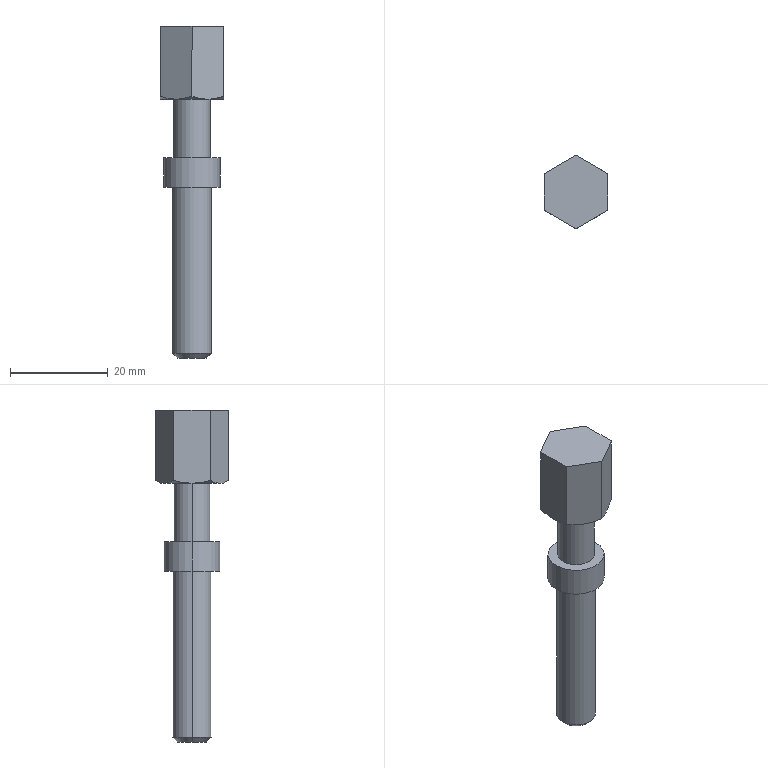Part | SolidWorks | features BaseBody 1 | 1 solid | 25 faces | box 13 x 15.011 x 68 mm | volume 5094 mm3 | plane 11 | cone 8 | cylinder 6 | commonest cylinder face diameters 7.5 x2 8 x2 11.5 x2
STEP:
#1=CARTESIAN_POINT('',(-4.,0.,-33.));
#2=VERTEX_POINT('',#1);
#3=CARTESIAN_POINT('',(4.,0.,-33.));
#4=VERTEX_POINT('',#3);
#5=CARTESIAN_POINT('',(0.,0.,-33.));
#6=DIRECTION('',(0.,0.,-1.));
#7=DIRECTION('',(-1.,0.,0.));
#8=AXIS2_PLACEMENT_3D('',#5,#6,#7);
#9=CIRCLE('',#8,4.);
#10=EDGE_CURVE('',#2,#4,#9,.T.);
#11=ORIENTED_EDGE('',*,*,#10,.T.);
#12=CARTESIAN_POINT('',(4.,0.,-67.));
#13=VERTEX_POINT('',#12);
#14=CARTESIAN_POINT('',(4.,0.,-68.));
#15=DIRECTION('',(0.,0.,-1.));
#16=VECTOR('',#15,1000.);
#17=LINE('',#14,#16);
#18=EDGE_CURVE('',#4,#13,#17,.T.);
#19=ORIENTED_EDGE('',*,*,#18,.T.);
#20=CARTESIAN_POINT('',(-4.,0.,-67.));
#21=VERTEX_POINT('',#20);
#22=CARTESIAN_POINT('',(0.,0.,-67.));
#23=DIRECTION('',(0.,0.,1.));
#24=DIRECTION('',(-1.,0.,0.));
#25=AXIS2_PLACEMENT_3D('',#22,#23,#24);
#26=CIRCLE('',#25,4.);
#27=EDGE_CURVE('',#13,#21,#26,.T.);
#28=ORIENTED_EDGE('',*,*,#27,.T.);
#29=CARTESIAN_POINT('',(-4.,0.,-68.));
#30=DIRECTION('',(0.,0.,-1.));
#31=VECTOR('',#30,1000.);
#32=LINE('',#29,#31);
#33=EDGE_CURVE('',#2,#21,#32,.T.);
#34=ORIENTED_EDGE('',*,*,#33,.F.);
#35=EDGE_LOOP('',(#11,#19,#28,#34));
#36=FACE_OUTER_BOUND('',#35,.T.);
#37=CARTESIAN_POINT('',(0.,0.,-68.));
#38=DIRECTION('',(0.,0.,-1.));
#39=DIRECTION('',(-1.,0.,0.));
#40=AXIS2_PLACEMENT_3D('',#37,#38,#39);
#41=CYLINDRICAL_SURFACE('',#40,4.);
#42=ADVANCED_FACE('',(#36),#41,.T.);
#43=CARTESIAN_POINT('',(3.,0.,-68.));
#44=VERTEX_POINT('',#43);
#45=CARTESIAN_POINT('',(-3.,0.,-68.));
#46=VERTEX_POINT('',#45);
#47=CARTESIAN_POINT('',(0.,0.,-68.));
#48=DIRECTION('',(0.,0.,1.));
#49=DIRECTION('',(1.,0.,0.));
#50=AXIS2_PLACEMENT_3D('',#47,#48,#49);
#51=CIRCLE('',#50,3.);
#52=EDGE_CURVE('',#44,#46,#51,.T.);
#53=ORIENTED_EDGE('',*,*,#52,.T.);
#54=CARTESIAN_POINT('',(-4.,0.,-67.));
#55=DIRECTION('',(-0.7071,0.,0.7071));
#56=VECTOR('',#55,1000.);
#57=LINE('',#54,#56);
#58=EDGE_CURVE('',#46,#21,#57,.T.);
#59=ORIENTED_EDGE('',*,*,#58,.T.);
#60=ORIENTED_EDGE('',*,*,#27,.F.);
#61=CARTESIAN_POINT('',(4.,0.,-67.));
#62=DIRECTION('',(0.7071,0.,0.7071));
#63=VECTOR('',#62,1000.);
#64=LINE('',#61,#63);
#65=EDGE_CURVE('',#44,#13,#64,.T.);
#66=ORIENTED_EDGE('',*,*,#65,.F.);
#67=EDGE_LOOP('',(#53,#59,#60,#66));
#68=FACE_OUTER_BOUND('',#67,.T.);
#69=CARTESIAN_POINT('',(0.,0.,-67.));
#70=DIRECTION('',(0.,0.,1.));
#71=DIRECTION('',(1.,0.,0.));
#72=AXIS2_PLACEMENT_3D('',#69,#70,#71);
#73=CONICAL_SURFACE('',#72,4.,0.7854);
#74=ADVANCED_FACE('',(#68),#73,.T.);
#75=CARTESIAN_POINT('',(-5.75,0.,-27.));
#76=VERTEX_POINT('',#75);
#77=CARTESIAN_POINT('',(5.75,0.,-27.));
#78=VERTEX_POINT('',#77);
#79=CARTESIAN_POINT('',(0.,0.,-27.));
#80=DIRECTION('',(0.,0.,-1.));
#81=DIRECTION('',(-1.,0.,0.));
#82=AXIS2_PLACEMENT_3D('',#79,#80,#81);
#83=CIRCLE('',#82,5.75);
#84=EDGE_CURVE('',#76,#78,#83,.T.);
#85=ORIENTED_EDGE('',*,*,#84,.T.);
#86=CARTESIAN_POINT('',(5.75,0.,-33.));
#87=VERTEX_POINT('',#86);
#88=CARTESIAN_POINT('',(5.75,0.,-68.));
#89=DIRECTION('',(0.,0.,-1.));
#90=VECTOR('',#89,1000.);
#91=LINE('',#88,#90);
#92=EDGE_CURVE('',#78,#87,#91,.T.);
#93=ORIENTED_EDGE('',*,*,#92,.T.);
#94=CARTESIAN_POINT('',(-5.75,0.,-33.));
#95=VERTEX_POINT('',#94);
#96=CARTESIAN_POINT('',(0.,0.,-33.));
#97=DIRECTION('',(0.,0.,1.));
#98=DIRECTION('',(-1.,0.,0.));
#99=AXIS2_PLACEMENT_3D('',#96,#97,#98);
#100=CIRCLE('',#99,5.75);
#101=EDGE_CURVE('',#87,#95,#100,.T.);
#102=ORIENTED_EDGE('',*,*,#101,.T.);
#103=CARTESIAN_POINT('',(-5.75,0.,-68.));
#104=DIRECTION('',(0.,0.,-1.));
#105=VECTOR('',#104,1000.);
#106=LINE('',#103,#105);
#107=EDGE_CURVE('',#76,#95,#106,.T.);
#108=ORIENTED_EDGE('',*,*,#107,.F.);
#109=EDGE_LOOP('',(#85,#93,#102,#108));
#110=FACE_OUTER_BOUND('',#109,.T.);
#111=CARTESIAN_POINT('',(0.,0.,-68.));
#112=DIRECTION('',(0.,0.,-1.));
#113=DIRECTION('',(-1.,0.,0.));
#114=AXIS2_PLACEMENT_3D('',#111,#112,#113);
#115=CYLINDRICAL_SURFACE('',#114,5.75);
#116=ADVANCED_FACE('',(#110),#115,.T.);
#117=CARTESIAN_POINT('',(-3.75,0.,-15.));
#118=VERTEX_POINT('',#117);
#119=CARTESIAN_POINT('',(3.75,0.,-15.));
#120=VERTEX_POINT('',#119);
#121=CARTESIAN_POINT('',(0.,0.,-15.));
#122=DIRECTION('',(0.,0.,-1.));
#123=DIRECTION('',(-1.,0.,0.));
#124=AXIS2_PLACEMENT_3D('',#121,#122,#123);
#125=CIRCLE('',#124,3.75);
#126=EDGE_CURVE('',#118,#120,#125,.T.);
#127=ORIENTED_EDGE('',*,*,#126,.T.);
#128=CARTESIAN_POINT('',(3.75,0.,-27.));
#129=VERTEX_POINT('',#128);
#130=CARTESIAN_POINT('',(3.75,0.,-68.));
#131=DIRECTION('',(0.,0.,-1.));
#132=VECTOR('',#131,1000.);
#133=LINE('',#130,#132);
#134=EDGE_CURVE('',#120,#129,#133,.T.);
#135=ORIENTED_EDGE('',*,*,#134,.T.);
#136=CARTESIAN_POINT('',(-3.75,0.,-27.));
#137=VERTEX_POINT('',#136);
#138=CARTESIAN_POINT('',(0.,0.,-27.));
#139=DIRECTION('',(0.,0.,1.));
#140=DIRECTION('',(-1.,0.,0.));
#141=AXIS2_PLACEMENT_3D('',#138,#139,#140);
#142=CIRCLE('',#141,3.75);
#143=EDGE_CURVE('',#129,#137,#142,.T.);
#144=ORIENTED_EDGE('',*,*,#143,.T.);
#145=CARTESIAN_POINT('',(-3.75,0.,-68.));
#146=DIRECTION('',(0.,0.,-1.));
#147=VECTOR('',#146,1000.);
#148=LINE('',#145,#147);
#149=EDGE_CURVE('',#118,#137,#148,.T.);
#150=ORIENTED_EDGE('',*,*,#149,.F.);
#151=EDGE_LOOP('',(#127,#135,#144,#150));
#152=FACE_OUTER_BOUND('',#151,.T.);
#153=CARTESIAN_POINT('',(0.,0.,-68.));
#154=DIRECTION('',(0.,0.,-1.));
#155=DIRECTION('',(-1.,0.,0.));
#156=AXIS2_PLACEMENT_3D('',#153,#154,#155);
#157=CYLINDRICAL_SURFACE('',#156,3.75);
#158=ADVANCED_FACE('',(#152),#157,.T.);
#159=ORIENTED_EDGE('',*,*,#18,.F.);
#160=CARTESIAN_POINT('',(0.,0.,-33.));
#161=DIRECTION('',(0.,0.,-1.));
#162=DIRECTION('',(-1.,0.,0.));
#163=AXIS2_PLACEMENT_3D('',#160,#161,#162);
#164=CIRCLE('',#163,4.);
#165=EDGE_CURVE('',#4,#2,#164,.T.);
#166=ORIENTED_EDGE('',*,*,#165,.T.);
#167=ORIENTED_EDGE('',*,*,#33,.T.);
#168=CARTESIAN_POINT('',(0.,0.,-67.));
#169=DIRECTION('',(0.,0.,1.));
#170=DIRECTION('',(-1.,0.,0.));
#171=AXIS2_PLACEMENT_3D('',#168,#169,#170);
#172=CIRCLE('',#171,4.);
#173=EDGE_CURVE('',#21,#13,#172,.T.);
#174=ORIENTED_EDGE('',*,*,#173,.T.);
#175=EDGE_LOOP('',(#159,#166,#167,#174));
#176=FACE_OUTER_BOUND('',#175,.T.);
#177=CARTESIAN_POINT('',(0.,0.,-68.));
#178=DIRECTION('',(0.,0.,-1.));
#179=DIRECTION('',(-1.,0.,0.));
#180=AXIS2_PLACEMENT_3D('',#177,#178,#179);
#181=CYLINDRICAL_SURFACE('',#180,4.);
#182=ADVANCED_FACE('',(#176),#181,.T.);
#183=CARTESIAN_POINT('',(0.,0.,-33.));
#184=DIRECTION('',(0.,0.,1.));
#185=DIRECTION('',(-1.,0.,0.));
#186=AXIS2_PLACEMENT_3D('',#183,#184,#185);
#187=CIRCLE('',#186,5.75);
#188=EDGE_CURVE('',#95,#87,#187,.T.);
#189=ORIENTED_EDGE('',*,*,#188,.F.);
#190=ORIENTED_EDGE('',*,*,#101,.F.);
#191=EDGE_LOOP('',(#189,#190));
#192=FACE_OUTER_BOUND('',#191,.T.);
#193=ORIENTED_EDGE('',*,*,#10,.F.);
#194=ORIENTED_EDGE('',*,*,#165,.F.);
#195=EDGE_LOOP('',(#193,#194));
#196=FACE_BOUND('',#195,.T.);
#197=CARTESIAN_POINT('',(0.,5.75,-33.));
#198=DIRECTION('',(0.,0.,1.));
#199=DIRECTION('',(1.,0.,0.));
#200=AXIS2_PLACEMENT_3D('',#197,#198,#199);
#201=PLANE('',#200);
#202=ADVANCED_FACE('',(#192,#196),#201,.F.);
#203=ORIENTED_EDGE('',*,*,#58,.F.);
#204=CARTESIAN_POINT('',(0.,0.,-68.));
#205=DIRECTION('',(0.,0.,1.));
#206=DIRECTION('',(1.,0.,0.));
#207=AXIS2_PLACEMENT_3D('',#204,#205,#206);
#208=CIRCLE('',#207,3.);
#209=EDGE_CURVE('',#46,#44,#208,.T.);
#210=ORIENTED_EDGE('',*,*,#209,.T.);
#211=ORIENTED_EDGE('',*,*,#65,.T.);
#212=ORIENTED_EDGE('',*,*,#173,.F.);
#213=EDGE_LOOP('',(#203,#210,#211,#212));
#214=FACE_OUTER_BOUND('',#213,.T.);
#215=CARTESIAN_POINT('',(0.,0.,-67.));
#216=DIRECTION('',(0.,0.,1.));
#217=DIRECTION('',(1.,0.,0.));
#218=AXIS2_PLACEMENT_3D('',#215,#216,#217);
#219=CONICAL_SURFACE('',#218,4.,0.7854);
#220=ADVANCED_FACE('',(#214),#219,.T.);
#221=ORIENTED_EDGE('',*,*,#92,.F.);
#222=CARTESIAN_POINT('',(0.,0.,-27.));
#223=DIRECTION('',(0.,0.,-1.));
#224=DIRECTION('',(-1.,0.,0.));
#225=AXIS2_PLACEMENT_3D('',#222,#223,#224);
#226=CIRCLE('',#225,5.75);
#227=EDGE_CURVE('',#78,#76,#226,.T.);
#228=ORIENTED_EDGE('',*,*,#227,.T.);
#229=ORIENTED_EDGE('',*,*,#107,.T.);
#230=ORIENTED_EDGE('',*,*,#188,.T.);
#231=EDGE_LOOP('',(#221,#228,#229,#230));
#232=FACE_OUTER_BOUND('',#231,.T.);
#233=CARTESIAN_POINT('',(0.,0.,-68.));
#234=DIRECTION('',(0.,0.,-1.));
#235=DIRECTION('',(-1.,0.,0.));
#236=AXIS2_PLACEMENT_3D('',#233,#234,#235);
#237=CYLINDRICAL_SURFACE('',#236,5.75);
#238=ADVANCED_FACE('',(#232),#237,.T.);
#239=ORIENTED_EDGE('',*,*,#52,.F.);
#240=ORIENTED_EDGE('',*,*,#209,.F.);
#241=EDGE_LOOP('',(#239,#240));
#242=FACE_OUTER_BOUND('',#241,.T.);
#243=CARTESIAN_POINT('',(0.,3.,-68.));
#244=DIRECTION('',(0.,0.,1.));
#245=DIRECTION('',(1.,0.,0.));
#246=AXIS2_PLACEMENT_3D('',#243,#244,#245);
#247=PLANE('',#246);
#248=ADVANCED_FACE('',(#242),#247,.F.);
#249=CARTESIAN_POINT('',(0.,0.,-27.));
#250=DIRECTION('',(0.,0.,1.));
#251=DIRECTION('',(-1.,0.,0.));
#252=AXIS2_PLACEMENT_3D('',#249,#250,#251);
#253=CIRCLE('',#252,3.75);
#254=EDGE_CURVE('',#137,#129,#253,.T.);
#255=ORIENTED_EDGE('',*,*,#254,.F.);
#256=ORIENTED_EDGE('',*,*,#143,.F.);
#257=EDGE_LOOP('',(#255,#256));
#258=FACE_BOUND('',#257,.T.);
#259=ORIENTED_EDGE('',*,*,#84,.F.);
#260=ORIENTED_EDGE('',*,*,#227,.F.);
#261=EDGE_LOOP('',(#259,#260));
#262=FACE_OUTER_BOUND('',#261,.T.);
#263=CARTESIAN_POINT('',(0.,3.75,-27.));
#264=DIRECTION('',(0.,0.,-1.));
#265=DIRECTION('',(-1.,0.,0.));
#266=AXIS2_PLACEMENT_3D('',#263,#264,#265);
#267=PLANE('',#266);
#268=ADVANCED_FACE('',(#258,#262),#267,.F.);
#269=ORIENTED_EDGE('',*,*,#134,.F.);
#270=CARTESIAN_POINT('',(0.,0.,-15.));
#271=DIRECTION('',(0.,0.,-1.));
#272=DIRECTION('',(-1.,0.,0.));
#273=AXIS2_PLACEMENT_3D('',#270,#271,#272);
#274=CIRCLE('',#273,3.75);
#275=EDGE_CURVE('',#120,#118,#274,.T.);
#276=ORIENTED_EDGE('',*,*,#275,.T.);
#277=ORIENTED_EDGE('',*,*,#149,.T.);
#278=ORIENTED_EDGE('',*,*,#254,.T.);
#279=EDGE_LOOP('',(#269,#276,#277,#278));
#280=FACE_OUTER_BOUND('',#279,.T.);
#281=CARTESIAN_POINT('',(0.,0.,-68.));
#282=DIRECTION('',(0.,0.,-1.));
#283=DIRECTION('',(-1.,0.,0.));
#284=AXIS2_PLACEMENT_3D('',#281,#282,#283);
#285=CYLINDRICAL_SURFACE('',#284,3.75);
#286=ADVANCED_FACE('',(#280),#285,.T.);
#287=CARTESIAN_POINT('',(-3.25,-5.629,-15.));
#288=VERTEX_POINT('',#287);
#289=CARTESIAN_POINT('',(3.25,-5.629,-15.));
#290=VERTEX_POINT('',#289);
#291=CARTESIAN_POINT('',(0.,0.,-15.));
#292=DIRECTION('',(0.,0.,1.));
#293=DIRECTION('',(1.,0.,0.));
#294=AXIS2_PLACEMENT_3D('',#291,#292,#293);
#295=CIRCLE('',#294,6.5);
#296=EDGE_CURVE('',#288,#290,#295,.T.);
#297=ORIENTED_EDGE('',*,*,#296,.F.);
#298=CARTESIAN_POINT('',(-6.5,0.,-15.));
#299=VERTEX_POINT('',#298);
#300=CARTESIAN_POINT('',(0.,0.,-15.));
#301=DIRECTION('',(0.,0.,1.));
#302=DIRECTION('',(0.,-1.,0.));
#303=AXIS2_PLACEMENT_3D('',#300,#301,#302);
#304=CIRCLE('',#303,6.5);
#305=EDGE_CURVE('',#299,#288,#304,.T.);
#306=ORIENTED_EDGE('',*,*,#305,.F.);
#307=CARTESIAN_POINT('',(-3.25,5.629,-15.));
#308=VERTEX_POINT('',#307);
#309=CARTESIAN_POINT('',(0.,0.,-15.));
#310=DIRECTION('',(0.,0.,1.));
#311=DIRECTION('',(0.,-1.,0.));
#312=AXIS2_PLACEMENT_3D('',#309,#310,#311);
#313=CIRCLE('',#312,6.5);
#314=EDGE_CURVE('',#308,#299,#313,.T.);
#315=ORIENTED_EDGE('',*,*,#314,.F.);
#316=CARTESIAN_POINT('',(3.25,5.629,-15.));
#317=VERTEX_POINT('',#316);
#318=CARTESIAN_POINT('',(0.,0.,-15.));
#319=DIRECTION('',(0.,0.,1.));
#320=DIRECTION('',(1.,0.,0.));
#321=AXIS2_PLACEMENT_3D('',#318,#319,#320);
#322=CIRCLE('',#321,6.5);
#323=EDGE_CURVE('',#317,#308,#322,.T.);
#324=ORIENTED_EDGE('',*,*,#323,.F.);
#325=CARTESIAN_POINT('',(6.5,0.,-15.));
#326=VERTEX_POINT('',#325);
#327=CARTESIAN_POINT('',(0.,0.,-15.));
#328=DIRECTION('',(0.,0.,1.));
#329=DIRECTION('',(0.,-1.,0.));
#330=AXIS2_PLACEMENT_3D('',#327,#328,#329);
#331=CIRCLE('',#330,6.5);
#332=EDGE_CURVE('',#326,#317,#331,.T.);
#333=ORIENTED_EDGE('',*,*,#332,.F.);
#334=CARTESIAN_POINT('',(0.,0.,-15.));
#335=DIRECTION('',(0.,0.,1.));
#336=DIRECTION('',(1.,0.,0.));
#337=AXIS2_PLACEMENT_3D('',#334,#335,#336);
#338=CIRCLE('',#337,6.5);
#339=EDGE_CURVE('',#290,#326,#338,.T.);
#340=ORIENTED_EDGE('',*,*,#339,.F.);
#341=EDGE_LOOP('',(#297,#306,#315,#324,#333,#340));
#342=FACE_OUTER_BOUND('',#341,.T.);
#343=ORIENTED_EDGE('',*,*,#126,.F.);
#344=ORIENTED_EDGE('',*,*,#275,.F.);
#345=EDGE_LOOP('',(#343,#344));
#346=FACE_BOUND('',#345,.T.);
#347=CARTESIAN_POINT('',(0.,0.,-15.));
#348=DIRECTION('',(0.,0.,1.));
#349=DIRECTION('',(1.,0.,0.));
#350=AXIS2_PLACEMENT_3D('',#347,#348,#349);
#351=PLANE('',#350);
#352=ADVANCED_FACE('',(#342,#346),#351,.F.);
#353=ORIENTED_EDGE('',*,*,#339,.T.);
#354=CARTESIAN_POINT('',(6.5,-3.753,-14.419));
#355=VERTEX_POINT('',#354);
#356=CARTESIAN_POINT('',(6.5,0.,-15.));
#357=CARTESIAN_POINT('',(6.5,-1.281,-15.));
#358=CARTESIAN_POINT('',(6.5,-2.527,-14.773));
#359=CARTESIAN_POINT('',(6.5,-3.753,-14.419));
#360=B_SPLINE_CURVE_WITH_KNOTS('',3,(#356,#357,#358,#359),.UNSPECIFIED.,.F.,.F.,(4,4),(0.,0.003797),.UNSPECIFIED.);
#361=EDGE_CURVE('',#326,#355,#360,.T.);
#362=ORIENTED_EDGE('',*,*,#361,.T.);
#363=CARTESIAN_POINT('',(6.5,-3.753,-14.419));
#364=CARTESIAN_POINT('',(5.438,-4.366,-14.773));
#365=CARTESIAN_POINT('',(4.359,-4.989,-15.));
#366=CARTESIAN_POINT('',(3.25,-5.629,-15.));
#367=B_SPLINE_CURVE_WITH_KNOTS('',3,(#363,#364,#365,#366),.UNSPECIFIED.,.F.,.F.,(4,4),(0.,0.003797),.UNSPECIFIED.);
#368=EDGE_CURVE('',#355,#290,#367,.T.);
#369=ORIENTED_EDGE('',*,*,#368,.T.);
#370=EDGE_LOOP('',(#353,#362,#369));
#371=FACE_OUTER_BOUND('',#370,.T.);
#372=CARTESIAN_POINT('',(0.,0.,-14.416));
#373=DIRECTION('',(0.,0.,1.));
#374=DIRECTION('',(1.,0.,0.));
#375=AXIS2_PLACEMENT_3D('',#372,#373,#374);
#376=CONICAL_SURFACE('',#375,7.512,1.047);
#377=ADVANCED_FACE('',(#371),#376,.T.);
#378=ORIENTED_EDGE('',*,*,#296,.T.);
#379=CARTESIAN_POINT('',(-0.000000043,-7.506,-14.419));
#380=VERTEX_POINT('',#379);
#381=CARTESIAN_POINT('',(3.25,-5.629,-15.));
#382=CARTESIAN_POINT('',(2.141,-6.27,-15.));
#383=CARTESIAN_POINT('',(1.062,-6.892,-14.773));
#384=CARTESIAN_POINT('',(-0.000000043,-7.506,-14.419));
#385=B_SPLINE_CURVE_WITH_KNOTS('',3,(#381,#382,#383,#384),.UNSPECIFIED.,.F.,.F.,(4,4),(0.,0.003797),.UNSPECIFIED.);
#386=EDGE_CURVE('',#290,#380,#385,.T.);
#387=ORIENTED_EDGE('',*,*,#386,.T.);
#388=CARTESIAN_POINT('',(-0.000000043,-7.506,-14.419));
#389=CARTESIAN_POINT('',(-1.062,-6.892,-14.773));
#390=CARTESIAN_POINT('',(-2.141,-6.27,-15.));
#391=CARTESIAN_POINT('',(-3.25,-5.629,-15.));
#392=B_SPLINE_CURVE_WITH_KNOTS('',3,(#388,#389,#390,#391),.UNSPECIFIED.,.F.,.F.,(4,4),(0.,0.003797),.UNSPECIFIED.);
#393=EDGE_CURVE('',#380,#288,#392,.T.);
#394=ORIENTED_EDGE('',*,*,#393,.T.);
#395=EDGE_LOOP('',(#378,#387,#394));
#396=FACE_OUTER_BOUND('',#395,.T.);
#397=CARTESIAN_POINT('',(0.,0.,-14.416));
#398=DIRECTION('',(0.,0.,1.));
#399=DIRECTION('',(1.,0.,0.));
#400=AXIS2_PLACEMENT_3D('',#397,#398,#399);
#401=CONICAL_SURFACE('',#400,7.512,1.047);
#402=ADVANCED_FACE('',(#396),#401,.T.);
#403=CARTESIAN_POINT('',(-6.5,-3.753,-14.419));
#404=VERTEX_POINT('',#403);
#405=CARTESIAN_POINT('',(-6.5,-3.753,-14.419));
#406=CARTESIAN_POINT('',(-6.5,-2.527,-14.773));
#407=CARTESIAN_POINT('',(-6.5,-1.281,-15.));
#408=CARTESIAN_POINT('',(-6.5,0.,-15.));
#409=B_SPLINE_CURVE_WITH_KNOTS('',3,(#405,#406,#407,#408),.UNSPECIFIED.,.F.,.F.,(4,4),(0.,0.003797),.UNSPECIFIED.);
#410=EDGE_CURVE('',#404,#299,#409,.T.);
#411=ORIENTED_EDGE('',*,*,#410,.T.);
#412=ORIENTED_EDGE('',*,*,#305,.T.);
#413=CARTESIAN_POINT('',(-3.25,-5.629,-15.));
#414=CARTESIAN_POINT('',(-4.359,-4.989,-15.));
#415=CARTESIAN_POINT('',(-5.438,-4.366,-14.773));
#416=CARTESIAN_POINT('',(-6.5,-3.753,-14.419));
#417=B_SPLINE_CURVE_WITH_KNOTS('',3,(#413,#414,#415,#416),.UNSPECIFIED.,.F.,.F.,(4,4),(0.,0.003797),.UNSPECIFIED.);
#418=EDGE_CURVE('',#288,#404,#417,.T.);
#419=ORIENTED_EDGE('',*,*,#418,.T.);
#420=EDGE_LOOP('',(#411,#412,#419));
#421=FACE_OUTER_BOUND('',#420,.T.);
#422=CARTESIAN_POINT('',(0.,0.,-14.416));
#423=DIRECTION('',(0.,0.,1.));
#424=DIRECTION('',(0.,-1.,0.));
#425=AXIS2_PLACEMENT_3D('',#422,#423,#424);
#426=CONICAL_SURFACE('',#425,7.512,1.047);
#427=ADVANCED_FACE('',(#421),#426,.T.);
#428=CARTESIAN_POINT('',(-6.5,3.753,-14.419));
#429=VERTEX_POINT('',#428);
#430=CARTESIAN_POINT('',(-6.5,3.753,-14.419));
#431=CARTESIAN_POINT('',(-5.438,4.366,-14.773));
#432=CARTESIAN_POINT('',(-4.359,4.989,-15.));
#433=CARTESIAN_POINT('',(-3.25,5.629,-15.));
#434=B_SPLINE_CURVE_WITH_KNOTS('',3,(#430,#431,#432,#433),.UNSPECIFIED.,.F.,.F.,(4,4),(0.,0.003797),.UNSPECIFIED.);
#435=EDGE_CURVE('',#429,#308,#434,.T.);
#436=ORIENTED_EDGE('',*,*,#435,.T.);
#437=ORIENTED_EDGE('',*,*,#314,.T.);
#438=CARTESIAN_POINT('',(-6.5,0.,-15.));
#439=CARTESIAN_POINT('',(-6.5,1.281,-15.));
#440=CARTESIAN_POINT('',(-6.5,2.527,-14.773));
#441=CARTESIAN_POINT('',(-6.5,3.753,-14.419));
#442=B_SPLINE_CURVE_WITH_KNOTS('',3,(#438,#439,#440,#441),.UNSPECIFIED.,.F.,.F.,(4,4),(0.,0.003797),.UNSPECIFIED.);
#443=EDGE_CURVE('',#299,#429,#442,.T.);
#444=ORIENTED_EDGE('',*,*,#443,.T.);
#445=EDGE_LOOP('',(#436,#437,#444));
#446=FACE_OUTER_BOUND('',#445,.T.);
#447=CARTESIAN_POINT('',(0.,0.,-14.416));
#448=DIRECTION('',(0.,0.,1.));
#449=DIRECTION('',(0.,-1.,0.));
#450=AXIS2_PLACEMENT_3D('',#447,#448,#449);
#451=CONICAL_SURFACE('',#450,7.512,1.047);
#452=ADVANCED_FACE('',(#446),#451,.T.);
#453=CARTESIAN_POINT('',(-0.000000029,7.506,-14.419));
#454=VERTEX_POINT('',#453);
#455=CARTESIAN_POINT('',(-0.000000029,7.506,-14.419));
#456=CARTESIAN_POINT('',(1.062,6.892,-14.773));
#457=CARTESIAN_POINT('',(2.141,6.27,-15.));
#458=CARTESIAN_POINT('',(3.25,5.629,-15.));
#459=B_SPLINE_CURVE_WITH_KNOTS('',3,(#455,#456,#457,#458),.UNSPECIFIED.,.F.,.F.,(4,4),(0.,0.003797),.UNSPECIFIED.);
#460=EDGE_CURVE('',#454,#317,#459,.T.);
#461=ORIENTED_EDGE('',*,*,#460,.T.);
#462=ORIENTED_EDGE('',*,*,#323,.T.);
#463=CARTESIAN_POINT('',(-3.25,5.629,-15.));
#464=CARTESIAN_POINT('',(-2.141,6.27,-15.));
#465=CARTESIAN_POINT('',(-1.062,6.892,-14.773));
#466=CARTESIAN_POINT('',(-0.000000029,7.506,-14.419));
#467=B_SPLINE_CURVE_WITH_KNOTS('',3,(#463,#464,#465,#466),.UNSPECIFIED.,.F.,.F.,(4,4),(0.,0.003797),.UNSPECIFIED.);
#468=EDGE_CURVE('',#308,#454,#467,.T.);
#469=ORIENTED_EDGE('',*,*,#468,.T.);
#470=EDGE_LOOP('',(#461,#462,#469));
#471=FACE_OUTER_BOUND('',#470,.T.);
#472=CARTESIAN_POINT('',(0.,0.,-14.416));
#473=DIRECTION('',(0.,0.,1.));
#474=DIRECTION('',(1.,0.,0.));
#475=AXIS2_PLACEMENT_3D('',#472,#473,#474);
#476=CONICAL_SURFACE('',#475,7.512,1.047);
#477=ADVANCED_FACE('',(#471),#476,.T.);
#478=ORIENTED_EDGE('',*,*,#332,.T.);
#479=CARTESIAN_POINT('',(6.5,3.753,-14.419));
#480=VERTEX_POINT('',#479);
#481=CARTESIAN_POINT('',(3.25,5.629,-15.));
#482=CARTESIAN_POINT('',(4.359,4.989,-15.));
#483=CARTESIAN_POINT('',(5.438,4.366,-14.773));
#484=CARTESIAN_POINT('',(6.5,3.753,-14.419));
#485=B_SPLINE_CURVE_WITH_KNOTS('',3,(#481,#482,#483,#484),.UNSPECIFIED.,.F.,.F.,(4,4),(0.,0.003797),.UNSPECIFIED.);
#486=EDGE_CURVE('',#317,#480,#485,.T.);
#487=ORIENTED_EDGE('',*,*,#486,.T.);
#488=CARTESIAN_POINT('',(6.5,3.753,-14.419));
#489=CARTESIAN_POINT('',(6.5,2.527,-14.773));
#490=CARTESIAN_POINT('',(6.5,1.281,-15.));
#491=CARTESIAN_POINT('',(6.5,0.,-15.));
#492=B_SPLINE_CURVE_WITH_KNOTS('',3,(#488,#489,#490,#491),.UNSPECIFIED.,.F.,.F.,(4,4),(0.,0.003797),.UNSPECIFIED.);
#493=EDGE_CURVE('',#480,#326,#492,.T.);
#494=ORIENTED_EDGE('',*,*,#493,.T.);
#495=EDGE_LOOP('',(#478,#487,#494));
#496=FACE_OUTER_BOUND('',#495,.T.);
#497=CARTESIAN_POINT('',(0.,0.,-14.416));
#498=DIRECTION('',(0.,0.,1.));
#499=DIRECTION('',(0.,-1.,0.));
#500=AXIS2_PLACEMENT_3D('',#497,#498,#499);
#501=CONICAL_SURFACE('',#500,7.512,1.047);
#502=ADVANCED_FACE('',(#496),#501,.T.);
#503=CARTESIAN_POINT('',(6.5,-3.753,0.));
#504=VERTEX_POINT('',#503);
#505=CARTESIAN_POINT('',(6.5,-3.753,-15.));
#506=DIRECTION('',(0.,0.,-1.));
#507=VECTOR('',#506,1000.);
#508=LINE('',#505,#507);
#509=EDGE_CURVE('',#504,#355,#508,.T.);
#510=ORIENTED_EDGE('',*,*,#509,.T.);
#511=ORIENTED_EDGE('',*,*,#361,.F.);
#512=ORIENTED_EDGE('',*,*,#493,.F.);
#513=CARTESIAN_POINT('',(6.5,3.753,0.));
#514=VERTEX_POINT('',#513);
#515=CARTESIAN_POINT('',(6.5,3.753,-15.));
#516=DIRECTION('',(0.,0.,1.));
#517=VECTOR('',#516,1000.);
#518=LINE('',#515,#517);
#519=EDGE_CURVE('',#480,#514,#518,.T.);
#520=ORIENTED_EDGE('',*,*,#519,.T.);
#521=CARTESIAN_POINT('',(6.5,-3.753,0.));
#522=DIRECTION('',(0.,-1.,0.));
#523=VECTOR('',#522,1000.);
#524=LINE('',#521,#523);
#525=EDGE_CURVE('',#514,#504,#524,.T.);
#526=ORIENTED_EDGE('',*,*,#525,.T.);
#527=EDGE_LOOP('',(#510,#511,#512,#520,#526));
#528=FACE_OUTER_BOUND('',#527,.T.);
#529=CARTESIAN_POINT('',(6.5,-3.753,-15.));
#530=DIRECTION('',(1.,0.,0.));
#531=DIRECTION('',(0.,0.,-1.));
#532=AXIS2_PLACEMENT_3D('',#529,#530,#531);
#533=PLANE('',#532);
#534=ADVANCED_FACE('',(#528),#533,.T.);
#535=CARTESIAN_POINT('',(0.,-7.506,0.));
#536=VERTEX_POINT('',#535);
#537=CARTESIAN_POINT('',(0.,-7.506,-15.));
#538=DIRECTION('',(0.,0.,-1.));
#539=VECTOR('',#538,1000.);
#540=LINE('',#537,#539);
#541=EDGE_CURVE('',#536,#380,#540,.T.);
#542=ORIENTED_EDGE('',*,*,#541,.T.);
#543=ORIENTED_EDGE('',*,*,#386,.F.);
#544=ORIENTED_EDGE('',*,*,#368,.F.);
#545=ORIENTED_EDGE('',*,*,#509,.F.);
#546=CARTESIAN_POINT('',(0.,-7.506,0.));
#547=DIRECTION('',(-0.866,-0.5,0.));
#548=VECTOR('',#547,1000.);
#549=LINE('',#546,#548);
#550=EDGE_CURVE('',#504,#536,#549,.T.);
#551=ORIENTED_EDGE('',*,*,#550,.T.);
#552=EDGE_LOOP('',(#542,#543,#544,#545,#551));
#553=FACE_OUTER_BOUND('',#552,.T.);
#554=CARTESIAN_POINT('',(0.,-7.506,-15.));
#555=DIRECTION('',(0.5,-0.866,0.));
#556=DIRECTION('',(0.866,0.5,0.));
#557=AXIS2_PLACEMENT_3D('',#554,#555,#556);
#558=PLANE('',#557);
#559=ADVANCED_FACE('',(#553),#558,.T.);
#560=CARTESIAN_POINT('',(-6.5,-3.753,0.));
#561=VERTEX_POINT('',#560);
#562=CARTESIAN_POINT('',(-6.5,-3.753,-15.));
#563=DIRECTION('',(0.,0.,-1.));
#564=VECTOR('',#563,1000.);
#565=LINE('',#562,#564);
#566=EDGE_CURVE('',#561,#404,#565,.T.);
#567=ORIENTED_EDGE('',*,*,#566,.T.);
#568=ORIENTED_EDGE('',*,*,#418,.F.);
#569=ORIENTED_EDGE('',*,*,#393,.F.);
#570=ORIENTED_EDGE('',*,*,#541,.F.);
#571=CARTESIAN_POINT('',(-6.5,-3.753,0.));
#572=DIRECTION('',(-0.866,0.5,0.));
#573=VECTOR('',#572,1000.);
#574=LINE('',#571,#573);
#575=EDGE_CURVE('',#536,#561,#574,.T.);
#576=ORIENTED_EDGE('',*,*,#575,.T.);
#577=EDGE_LOOP('',(#567,#568,#569,#570,#576));
#578=FACE_OUTER_BOUND('',#577,.T.);
#579=CARTESIAN_POINT('',(-6.5,-3.753,-15.));
#580=DIRECTION('',(-0.5,-0.866,0.));
#581=DIRECTION('',(0.866,-0.5,0.));
#582=AXIS2_PLACEMENT_3D('',#579,#580,#581);
#583=PLANE('',#582);
#584=ADVANCED_FACE('',(#578),#583,.T.);
#585=CARTESIAN_POINT('',(-6.5,3.753,0.));
#586=VERTEX_POINT('',#585);
#587=CARTESIAN_POINT('',(-6.5,3.753,-15.));
#588=DIRECTION('',(0.,0.,-1.));
#589=VECTOR('',#588,1000.);
#590=LINE('',#587,#589);
#591=EDGE_CURVE('',#586,#429,#590,.T.);
#592=ORIENTED_EDGE('',*,*,#591,.T.);
#593=ORIENTED_EDGE('',*,*,#443,.F.);
#594=ORIENTED_EDGE('',*,*,#410,.F.);
#595=ORIENTED_EDGE('',*,*,#566,.F.);
#596=CARTESIAN_POINT('',(-6.5,3.753,0.));
#597=DIRECTION('',(0.,1.,0.));
#598=VECTOR('',#597,1000.);
#599=LINE('',#596,#598);
#600=EDGE_CURVE('',#561,#586,#599,.T.);
#601=ORIENTED_EDGE('',*,*,#600,.T.);
#602=EDGE_LOOP('',(#592,#593,#594,#595,#601));
#603=FACE_OUTER_BOUND('',#602,.T.);
#604=CARTESIAN_POINT('',(-6.5,3.753,-15.));
#605=DIRECTION('',(-1.,0.,0.));
#606=DIRECTION('',(0.,0.,1.));
#607=AXIS2_PLACEMENT_3D('',#604,#605,#606);
#608=PLANE('',#607);
#609=ADVANCED_FACE('',(#603),#608,.T.);
#610=CARTESIAN_POINT('',(0.,7.506,0.));
#611=VERTEX_POINT('',#610);
#612=CARTESIAN_POINT('',(0.,7.506,-15.));
#613=DIRECTION('',(0.,0.,-1.));
#614=VECTOR('',#613,1000.);
#615=LINE('',#612,#614);
#616=EDGE_CURVE('',#611,#454,#615,.T.);
#617=ORIENTED_EDGE('',*,*,#616,.T.);
#618=ORIENTED_EDGE('',*,*,#468,.F.);
#619=ORIENTED_EDGE('',*,*,#435,.F.);
#620=ORIENTED_EDGE('',*,*,#591,.F.);
#621=CARTESIAN_POINT('',(0.,7.506,0.));
#622=DIRECTION('',(0.866,0.5,0.));
#623=VECTOR('',#622,1000.);
#624=LINE('',#621,#623);
#625=EDGE_CURVE('',#586,#611,#624,.T.);
#626=ORIENTED_EDGE('',*,*,#625,.T.);
#627=EDGE_LOOP('',(#617,#618,#619,#620,#626));
#628=FACE_OUTER_BOUND('',#627,.T.);
#629=CARTESIAN_POINT('',(0.,7.506,-15.));
#630=DIRECTION('',(-0.5,0.866,0.));
#631=DIRECTION('',(-0.866,-0.5,0.));
#632=AXIS2_PLACEMENT_3D('',#629,#630,#631);
#633=PLANE('',#632);
#634=ADVANCED_FACE('',(#628),#633,.T.);
#635=ORIENTED_EDGE('',*,*,#519,.F.);
#636=ORIENTED_EDGE('',*,*,#486,.F.);
#637=ORIENTED_EDGE('',*,*,#460,.F.);
#638=ORIENTED_EDGE('',*,*,#616,.F.);
#639=CARTESIAN_POINT('',(6.5,3.753,0.));
#640=DIRECTION('',(0.866,-0.5,0.));
#641=VECTOR('',#640,1000.);
#642=LINE('',#639,#641);
#643=EDGE_CURVE('',#611,#514,#642,.T.);
#644=ORIENTED_EDGE('',*,*,#643,.T.);
#645=EDGE_LOOP('',(#635,#636,#637,#638,#644));
#646=FACE_OUTER_BOUND('',#645,.T.);
#647=CARTESIAN_POINT('',(6.5,3.753,-15.));
#648=DIRECTION('',(0.5,0.866,0.));
#649=DIRECTION('',(-0.866,0.5,0.));
#650=AXIS2_PLACEMENT_3D('',#647,#648,#649);
#651=PLANE('',#650);
#652=ADVANCED_FACE('',(#646),#651,.T.);
#653=ORIENTED_EDGE('',*,*,#525,.F.);
#654=ORIENTED_EDGE('',*,*,#643,.F.);
#655=ORIENTED_EDGE('',*,*,#625,.F.);
#656=ORIENTED_EDGE('',*,*,#600,.F.);
#657=ORIENTED_EDGE('',*,*,#575,.F.);
#658=ORIENTED_EDGE('',*,*,#550,.F.);
#659=EDGE_LOOP('',(#653,#654,#655,#656,#657,#658));
#660=FACE_OUTER_BOUND('',#659,.T.);
#661=CARTESIAN_POINT('',(0.,0.,0.));
#662=DIRECTION('',(0.,0.,1.));
#663=DIRECTION('',(1.,0.,0.));
#664=AXIS2_PLACEMENT_3D('',#661,#662,#663);
#665=PLANE('',#664);
#666=ADVANCED_FACE('',(#660),#665,.T.);
#667=CLOSED_SHELL('',(#42,#74,#116,#158,#182,#202,#220,#238,#248,#268,#286,#352,#377,#402,#427,#452,#477,#502,#534,#559,#584,#609,#634,#652,#666));
#668=MANIFOLD_SOLID_BREP('',#667);
#669=CARTESIAN_POINT('',(0.,0.,0.));
#670=DIRECTION('',(0.,0.,1.));
#671=DIRECTION('',(1.,0.,0.));
#672=AXIS2_PLACEMENT_3D('',#669,#670,#671);
#673=(LENGTH_UNIT()NAMED_UNIT(*)SI_UNIT(.MILLI.,.METRE.));
#674=UNCERTAINTY_MEASURE_WITH_UNIT(LENGTH_MEASURE(0.00001),#673,'','');
#675=(NAMED_UNIT(*)PLANE_ANGLE_UNIT()SI_UNIT($,.RADIAN.));
#676=(NAMED_UNIT(*)SI_UNIT($,.STERADIAN.)SOLID_ANGLE_UNIT());
#677=(GEOMETRIC_REPRESENTATION_CONTEXT(3)GLOBAL_UNCERTAINTY_ASSIGNED_CONTEXT((#674))GLOBAL_UNIT_ASSIGNED_CONTEXT((#673,#675,#676))REPRESENTATION_CONTEXT('',''));
#678=ADVANCED_BREP_SHAPE_REPRESENTATION('',(#668,#672),#677);